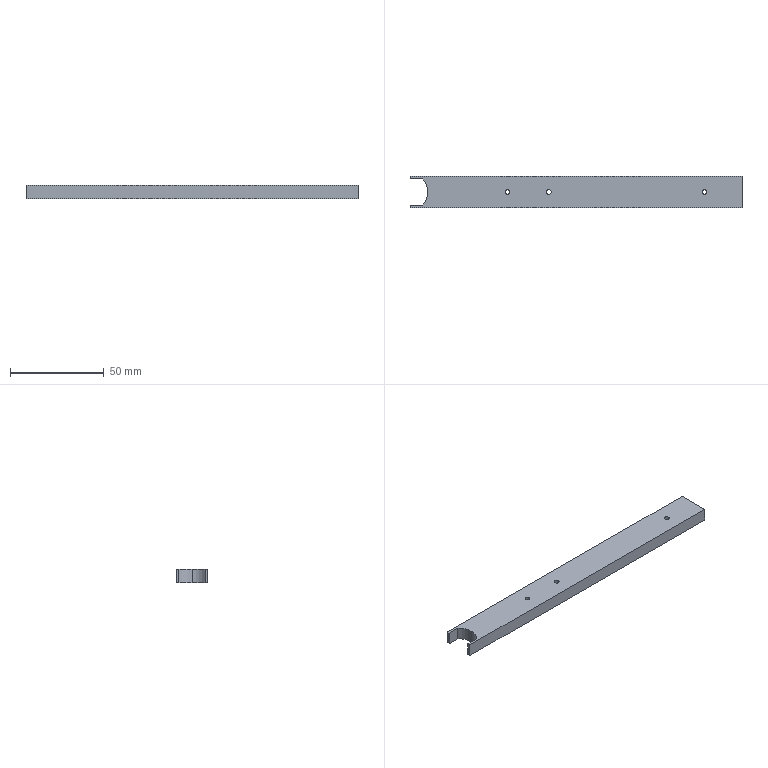Part | STEP file | BU-D02-2a#180 | 1 solid | 17 faces | box 177 x 17 x 7 mm | volume 20122 mm3 | plane 9 | cylinder 8 | commonest cylinder face diameters 2.5 x6 19 x2
STEP:
#1=CARTESIAN_POINT('',(0.,0.,0.));
#2=DIRECTION('',(0.,0.,1.));
#3=DIRECTION('',(1.,0.,0.));
#4=AXIS2_PLACEMENT_3D('',#1,#2,#3);
#5=CARTESIAN_POINT('',(53.25,0.,0.));
#6=VERTEX_POINT('',#5);
#7=CARTESIAN_POINT('',(53.25,0.,7.));
#8=VERTEX_POINT('',#7);
#9=CARTESIAN_POINT('',(53.25,0.,7.));
#10=DIRECTION('',(0.,0.,1.));
#11=VECTOR('',#10,1.);
#12=LINE('',#9,#11);
#13=CARTESIAN_POINT('',(52.,0.,7.));
#14=DIRECTION('',(0.,0.,1.));
#15=DIRECTION('',(1.,0.,0.));
#16=AXIS2_PLACEMENT_3D('',#13,#14,#15);
#17=CYLINDRICAL_SURFACE('',#16,1.25);
#18=CARTESIAN_POINT('',(6.283,0.));
#19=DIRECTION('',(0.,1.));
#20=VECTOR('',#19,1.);
#21=LINE('',#18,#20);
#22=(GEOMETRIC_REPRESENTATION_CONTEXT(2)PARAMETRIC_REPRESENTATION_CONTEXT()REPRESENTATION_CONTEXT('',''));
#23=DEFINITIONAL_REPRESENTATION('',(#21),#22);
#24=PCURVE('',#17,#23);
#25=CARTESIAN_POINT('',(52.,0.,7.));
#26=DIRECTION('',(0.,0.,1.));
#27=DIRECTION('',(1.,0.,0.));
#28=AXIS2_PLACEMENT_3D('',#25,#26,#27);
#29=CYLINDRICAL_SURFACE('',#28,1.25);
#30=CARTESIAN_POINT('',(0.,0.));
#31=DIRECTION('',(0.,1.));
#32=VECTOR('',#31,1.);
#33=LINE('',#30,#32);
#34=(GEOMETRIC_REPRESENTATION_CONTEXT(2)PARAMETRIC_REPRESENTATION_CONTEXT()REPRESENTATION_CONTEXT('',''));
#35=DEFINITIONAL_REPRESENTATION('',(#33),#34);
#36=PCURVE('',#29,#35);
#37=SURFACE_CURVE('',#12,(#24,#36),.PCURVE_S1.);
#38=EDGE_CURVE('',#6,#8,#37,.T.);
#39=ORIENTED_EDGE('',*,*,#38,.T.);
#40=CARTESIAN_POINT('',(50.75,0.,7.));
#41=VERTEX_POINT('',#40);
#42=CARTESIAN_POINT('',(52.,0.,7.));
#43=DIRECTION('',(0.,0.,1.));
#44=DIRECTION('',(1.,0.,0.));
#45=AXIS2_PLACEMENT_3D('',#42,#43,#44);
#46=CIRCLE('',#45,1.25);
#47=CARTESIAN_POINT('',(0.,0.));
#48=DIRECTION('',(1.,0.));
#49=VECTOR('',#48,1.);
#50=LINE('',#47,#49);
#51=(GEOMETRIC_REPRESENTATION_CONTEXT(2)PARAMETRIC_REPRESENTATION_CONTEXT()REPRESENTATION_CONTEXT('',''));
#52=DEFINITIONAL_REPRESENTATION('',(#50),#51);
#53=PCURVE('',#17,#52);
#54=CARTESIAN_POINT('',(0.,0.,7.));
#55=DIRECTION('',(0.,0.,1.));
#56=DIRECTION('',(1.,0.,0.));
#57=AXIS2_PLACEMENT_3D('',#54,#55,#56);
#58=PLANE('',#57);
#59=CARTESIAN_POINT('',(52.,0.));
#60=DIRECTION('',(1.,0.));
#61=AXIS2_PLACEMENT_2D('',#59,#60);
#62=CIRCLE('',#61,1.25);
#63=(GEOMETRIC_REPRESENTATION_CONTEXT(2)PARAMETRIC_REPRESENTATION_CONTEXT()REPRESENTATION_CONTEXT('',''));
#64=DEFINITIONAL_REPRESENTATION('',(#62),#63);
#65=PCURVE('',#58,#64);
#66=SURFACE_CURVE('',#46,(#53,#65),.PCURVE_S1.);
#67=EDGE_CURVE('',#41,#8,#66,.T.);
#68=ORIENTED_EDGE('',*,*,#67,.F.);
#69=CARTESIAN_POINT('',(50.75,0.,0.));
#70=VERTEX_POINT('',#69);
#71=CARTESIAN_POINT('',(50.75,0.,7.));
#72=DIRECTION('',(0.,0.,1.));
#73=VECTOR('',#72,1.);
#74=LINE('',#71,#73);
#75=CARTESIAN_POINT('',(3.142,0.));
#76=DIRECTION('',(0.,1.));
#77=VECTOR('',#76,1.);
#78=LINE('',#75,#77);
#79=(GEOMETRIC_REPRESENTATION_CONTEXT(2)PARAMETRIC_REPRESENTATION_CONTEXT()REPRESENTATION_CONTEXT('',''));
#80=DEFINITIONAL_REPRESENTATION('',(#78),#79);
#81=PCURVE('',#17,#80);
#82=CARTESIAN_POINT('',(3.142,0.));
#83=DIRECTION('',(0.,1.));
#84=VECTOR('',#83,1.);
#85=LINE('',#82,#84);
#86=(GEOMETRIC_REPRESENTATION_CONTEXT(2)PARAMETRIC_REPRESENTATION_CONTEXT()REPRESENTATION_CONTEXT('',''));
#87=DEFINITIONAL_REPRESENTATION('',(#85),#86);
#88=PCURVE('',#29,#87);
#89=SURFACE_CURVE('',#74,(#81,#88),.PCURVE_S1.);
#90=EDGE_CURVE('',#70,#41,#89,.T.);
#91=ORIENTED_EDGE('',*,*,#90,.F.);
#92=CARTESIAN_POINT('',(52.,0.,0.));
#93=DIRECTION('',(0.,0.,1.));
#94=DIRECTION('',(1.,0.,0.));
#95=AXIS2_PLACEMENT_3D('',#92,#93,#94);
#96=CIRCLE('',#95,1.25);
#97=CARTESIAN_POINT('',(0.,-7.));
#98=DIRECTION('',(1.,0.));
#99=VECTOR('',#98,1.);
#100=LINE('',#97,#99);
#101=(GEOMETRIC_REPRESENTATION_CONTEXT(2)PARAMETRIC_REPRESENTATION_CONTEXT()REPRESENTATION_CONTEXT('',''));
#102=DEFINITIONAL_REPRESENTATION('',(#100),#101);
#103=PCURVE('',#17,#102);
#104=CARTESIAN_POINT('',(0.,0.,0.));
#105=DIRECTION('',(0.,0.,1.));
#106=DIRECTION('',(1.,0.,0.));
#107=AXIS2_PLACEMENT_3D('',#104,#105,#106);
#108=PLANE('',#107);
#109=CARTESIAN_POINT('',(52.,0.));
#110=DIRECTION('',(1.,0.));
#111=AXIS2_PLACEMENT_2D('',#109,#110);
#112=CIRCLE('',#111,1.25);
#113=(GEOMETRIC_REPRESENTATION_CONTEXT(2)PARAMETRIC_REPRESENTATION_CONTEXT()REPRESENTATION_CONTEXT('',''));
#114=DEFINITIONAL_REPRESENTATION('',(#112),#113);
#115=PCURVE('',#108,#114);
#116=SURFACE_CURVE('',#96,(#103,#115),.PCURVE_S1.);
#117=EDGE_CURVE('',#70,#6,#116,.T.);
#118=ORIENTED_EDGE('',*,*,#117,.T.);
#119=EDGE_LOOP('',(#39,#68,#91,#118));
#120=FACE_BOUND('',#119,.F.);
#121=ADVANCED_FACE('',(#120),#17,.F.);
#122=CARTESIAN_POINT('',(75.25,0.,0.));
#123=VERTEX_POINT('',#122);
#124=CARTESIAN_POINT('',(75.25,0.,7.));
#125=VERTEX_POINT('',#124);
#126=CARTESIAN_POINT('',(75.25,0.,7.));
#127=DIRECTION('',(0.,0.,1.));
#128=VECTOR('',#127,1.);
#129=LINE('',#126,#128);
#130=CARTESIAN_POINT('',(74.,0.,7.));
#131=DIRECTION('',(0.,0.,1.));
#132=DIRECTION('',(1.,0.,0.));
#133=AXIS2_PLACEMENT_3D('',#130,#131,#132);
#134=CYLINDRICAL_SURFACE('',#133,1.25);
#135=CARTESIAN_POINT('',(6.283,0.));
#136=DIRECTION('',(0.,1.));
#137=VECTOR('',#136,1.);
#138=LINE('',#135,#137);
#139=(GEOMETRIC_REPRESENTATION_CONTEXT(2)PARAMETRIC_REPRESENTATION_CONTEXT()REPRESENTATION_CONTEXT('',''));
#140=DEFINITIONAL_REPRESENTATION('',(#138),#139);
#141=PCURVE('',#134,#140);
#142=CARTESIAN_POINT('',(74.,0.,7.));
#143=DIRECTION('',(0.,0.,1.));
#144=DIRECTION('',(1.,0.,0.));
#145=AXIS2_PLACEMENT_3D('',#142,#143,#144);
#146=CYLINDRICAL_SURFACE('',#145,1.25);
#147=CARTESIAN_POINT('',(0.,0.));
#148=DIRECTION('',(0.,1.));
#149=VECTOR('',#148,1.);
#150=LINE('',#147,#149);
#151=(GEOMETRIC_REPRESENTATION_CONTEXT(2)PARAMETRIC_REPRESENTATION_CONTEXT()REPRESENTATION_CONTEXT('',''));
#152=DEFINITIONAL_REPRESENTATION('',(#150),#151);
#153=PCURVE('',#146,#152);
#154=SURFACE_CURVE('',#129,(#141,#153),.PCURVE_S1.);
#155=EDGE_CURVE('',#123,#125,#154,.T.);
#156=ORIENTED_EDGE('',*,*,#155,.T.);
#157=CARTESIAN_POINT('',(72.75,0.,7.));
#158=VERTEX_POINT('',#157);
#159=CARTESIAN_POINT('',(74.,0.,7.));
#160=DIRECTION('',(0.,0.,1.));
#161=DIRECTION('',(1.,0.,0.));
#162=AXIS2_PLACEMENT_3D('',#159,#160,#161);
#163=CIRCLE('',#162,1.25);
#164=CARTESIAN_POINT('',(0.,0.));
#165=DIRECTION('',(1.,0.));
#166=VECTOR('',#165,1.);
#167=LINE('',#164,#166);
#168=(GEOMETRIC_REPRESENTATION_CONTEXT(2)PARAMETRIC_REPRESENTATION_CONTEXT()REPRESENTATION_CONTEXT('',''));
#169=DEFINITIONAL_REPRESENTATION('',(#167),#168);
#170=PCURVE('',#134,#169);
#171=CARTESIAN_POINT('',(74.,0.));
#172=DIRECTION('',(1.,0.));
#173=AXIS2_PLACEMENT_2D('',#171,#172);
#174=CIRCLE('',#173,1.25);
#175=(GEOMETRIC_REPRESENTATION_CONTEXT(2)PARAMETRIC_REPRESENTATION_CONTEXT()REPRESENTATION_CONTEXT('',''));
#176=DEFINITIONAL_REPRESENTATION('',(#174),#175);
#177=PCURVE('',#58,#176);
#178=SURFACE_CURVE('',#163,(#170,#177),.PCURVE_S1.);
#179=EDGE_CURVE('',#158,#125,#178,.T.);
#180=ORIENTED_EDGE('',*,*,#179,.F.);
#181=CARTESIAN_POINT('',(72.75,0.,0.));
#182=VERTEX_POINT('',#181);
#183=CARTESIAN_POINT('',(72.75,0.,7.));
#184=DIRECTION('',(0.,0.,1.));
#185=VECTOR('',#184,1.);
#186=LINE('',#183,#185);
#187=CARTESIAN_POINT('',(3.142,0.));
#188=DIRECTION('',(0.,1.));
#189=VECTOR('',#188,1.);
#190=LINE('',#187,#189);
#191=(GEOMETRIC_REPRESENTATION_CONTEXT(2)PARAMETRIC_REPRESENTATION_CONTEXT()REPRESENTATION_CONTEXT('',''));
#192=DEFINITIONAL_REPRESENTATION('',(#190),#191);
#193=PCURVE('',#134,#192);
#194=CARTESIAN_POINT('',(3.142,0.));
#195=DIRECTION('',(0.,1.));
#196=VECTOR('',#195,1.);
#197=LINE('',#194,#196);
#198=(GEOMETRIC_REPRESENTATION_CONTEXT(2)PARAMETRIC_REPRESENTATION_CONTEXT()REPRESENTATION_CONTEXT('',''));
#199=DEFINITIONAL_REPRESENTATION('',(#197),#198);
#200=PCURVE('',#146,#199);
#201=SURFACE_CURVE('',#186,(#193,#200),.PCURVE_S1.);
#202=EDGE_CURVE('',#182,#158,#201,.T.);
#203=ORIENTED_EDGE('',*,*,#202,.F.);
#204=CARTESIAN_POINT('',(74.,0.,0.));
#205=DIRECTION('',(0.,0.,1.));
#206=DIRECTION('',(1.,0.,0.));
#207=AXIS2_PLACEMENT_3D('',#204,#205,#206);
#208=CIRCLE('',#207,1.25);
#209=CARTESIAN_POINT('',(0.,-7.));
#210=DIRECTION('',(1.,0.));
#211=VECTOR('',#210,1.);
#212=LINE('',#209,#211);
#213=(GEOMETRIC_REPRESENTATION_CONTEXT(2)PARAMETRIC_REPRESENTATION_CONTEXT()REPRESENTATION_CONTEXT('',''));
#214=DEFINITIONAL_REPRESENTATION('',(#212),#213);
#215=PCURVE('',#134,#214);
#216=CARTESIAN_POINT('',(74.,0.));
#217=DIRECTION('',(1.,0.));
#218=AXIS2_PLACEMENT_2D('',#216,#217);
#219=CIRCLE('',#218,1.25);
#220=(GEOMETRIC_REPRESENTATION_CONTEXT(2)PARAMETRIC_REPRESENTATION_CONTEXT()REPRESENTATION_CONTEXT('',''));
#221=DEFINITIONAL_REPRESENTATION('',(#219),#220);
#222=PCURVE('',#108,#221);
#223=SURFACE_CURVE('',#208,(#215,#222),.PCURVE_S1.);
#224=EDGE_CURVE('',#182,#123,#223,.T.);
#225=ORIENTED_EDGE('',*,*,#224,.T.);
#226=EDGE_LOOP('',(#156,#180,#203,#225));
#227=FACE_BOUND('',#226,.F.);
#228=ADVANCED_FACE('',(#227),#134,.F.);
#229=CARTESIAN_POINT('',(158.25,0.,0.));
#230=VERTEX_POINT('',#229);
#231=CARTESIAN_POINT('',(158.25,0.,7.));
#232=VERTEX_POINT('',#231);
#233=CARTESIAN_POINT('',(158.25,0.,7.));
#234=DIRECTION('',(0.,0.,1.));
#235=VECTOR('',#234,1.);
#236=LINE('',#233,#235);
#237=CARTESIAN_POINT('',(157.,0.,7.));
#238=DIRECTION('',(0.,0.,1.));
#239=DIRECTION('',(1.,0.,0.));
#240=AXIS2_PLACEMENT_3D('',#237,#238,#239);
#241=CYLINDRICAL_SURFACE('',#240,1.25);
#242=CARTESIAN_POINT('',(6.283,0.));
#243=DIRECTION('',(0.,1.));
#244=VECTOR('',#243,1.);
#245=LINE('',#242,#244);
#246=(GEOMETRIC_REPRESENTATION_CONTEXT(2)PARAMETRIC_REPRESENTATION_CONTEXT()REPRESENTATION_CONTEXT('',''));
#247=DEFINITIONAL_REPRESENTATION('',(#245),#246);
#248=PCURVE('',#241,#247);
#249=CARTESIAN_POINT('',(157.,0.,7.));
#250=DIRECTION('',(0.,0.,1.));
#251=DIRECTION('',(1.,0.,0.));
#252=AXIS2_PLACEMENT_3D('',#249,#250,#251);
#253=CYLINDRICAL_SURFACE('',#252,1.25);
#254=CARTESIAN_POINT('',(0.,0.));
#255=DIRECTION('',(0.,1.));
#256=VECTOR('',#255,1.);
#257=LINE('',#254,#256);
#258=(GEOMETRIC_REPRESENTATION_CONTEXT(2)PARAMETRIC_REPRESENTATION_CONTEXT()REPRESENTATION_CONTEXT('',''));
#259=DEFINITIONAL_REPRESENTATION('',(#257),#258);
#260=PCURVE('',#253,#259);
#261=SURFACE_CURVE('',#236,(#248,#260),.PCURVE_S1.);
#262=EDGE_CURVE('',#230,#232,#261,.T.);
#263=ORIENTED_EDGE('',*,*,#262,.T.);
#264=CARTESIAN_POINT('',(155.75,0.,7.));
#265=VERTEX_POINT('',#264);
#266=CARTESIAN_POINT('',(157.,0.,7.));
#267=DIRECTION('',(0.,0.,1.));
#268=DIRECTION('',(1.,0.,0.));
#269=AXIS2_PLACEMENT_3D('',#266,#267,#268);
#270=CIRCLE('',#269,1.25);
#271=CARTESIAN_POINT('',(0.,0.));
#272=DIRECTION('',(1.,0.));
#273=VECTOR('',#272,1.);
#274=LINE('',#271,#273);
#275=(GEOMETRIC_REPRESENTATION_CONTEXT(2)PARAMETRIC_REPRESENTATION_CONTEXT()REPRESENTATION_CONTEXT('',''));
#276=DEFINITIONAL_REPRESENTATION('',(#274),#275);
#277=PCURVE('',#241,#276);
#278=CARTESIAN_POINT('',(157.,0.));
#279=DIRECTION('',(1.,0.));
#280=AXIS2_PLACEMENT_2D('',#278,#279);
#281=CIRCLE('',#280,1.25);
#282=(GEOMETRIC_REPRESENTATION_CONTEXT(2)PARAMETRIC_REPRESENTATION_CONTEXT()REPRESENTATION_CONTEXT('',''));
#283=DEFINITIONAL_REPRESENTATION('',(#281),#282);
#284=PCURVE('',#58,#283);
#285=SURFACE_CURVE('',#270,(#277,#284),.PCURVE_S1.);
#286=EDGE_CURVE('',#265,#232,#285,.T.);
#287=ORIENTED_EDGE('',*,*,#286,.F.);
#288=CARTESIAN_POINT('',(155.75,0.,0.));
#289=VERTEX_POINT('',#288);
#290=CARTESIAN_POINT('',(155.75,0.,7.));
#291=DIRECTION('',(0.,0.,1.));
#292=VECTOR('',#291,1.);
#293=LINE('',#290,#292);
#294=CARTESIAN_POINT('',(3.142,0.));
#295=DIRECTION('',(0.,1.));
#296=VECTOR('',#295,1.);
#297=LINE('',#294,#296);
#298=(GEOMETRIC_REPRESENTATION_CONTEXT(2)PARAMETRIC_REPRESENTATION_CONTEXT()REPRESENTATION_CONTEXT('',''));
#299=DEFINITIONAL_REPRESENTATION('',(#297),#298);
#300=PCURVE('',#241,#299);
#301=CARTESIAN_POINT('',(3.142,0.));
#302=DIRECTION('',(0.,1.));
#303=VECTOR('',#302,1.);
#304=LINE('',#301,#303);
#305=(GEOMETRIC_REPRESENTATION_CONTEXT(2)PARAMETRIC_REPRESENTATION_CONTEXT()REPRESENTATION_CONTEXT('',''));
#306=DEFINITIONAL_REPRESENTATION('',(#304),#305);
#307=PCURVE('',#253,#306);
#308=SURFACE_CURVE('',#293,(#300,#307),.PCURVE_S1.);
#309=EDGE_CURVE('',#289,#265,#308,.T.);
#310=ORIENTED_EDGE('',*,*,#309,.F.);
#311=CARTESIAN_POINT('',(157.,0.,0.));
#312=DIRECTION('',(0.,0.,1.));
#313=DIRECTION('',(1.,0.,0.));
#314=AXIS2_PLACEMENT_3D('',#311,#312,#313);
#315=CIRCLE('',#314,1.25);
#316=CARTESIAN_POINT('',(0.,-7.));
#317=DIRECTION('',(1.,0.));
#318=VECTOR('',#317,1.);
#319=LINE('',#316,#318);
#320=(GEOMETRIC_REPRESENTATION_CONTEXT(2)PARAMETRIC_REPRESENTATION_CONTEXT()REPRESENTATION_CONTEXT('',''));
#321=DEFINITIONAL_REPRESENTATION('',(#319),#320);
#322=PCURVE('',#241,#321);
#323=CARTESIAN_POINT('',(157.,0.));
#324=DIRECTION('',(1.,0.));
#325=AXIS2_PLACEMENT_2D('',#323,#324);
#326=CIRCLE('',#325,1.25);
#327=(GEOMETRIC_REPRESENTATION_CONTEXT(2)PARAMETRIC_REPRESENTATION_CONTEXT()REPRESENTATION_CONTEXT('',''));
#328=DEFINITIONAL_REPRESENTATION('',(#326),#327);
#329=PCURVE('',#108,#328);
#330=SURFACE_CURVE('',#315,(#322,#329),.PCURVE_S1.);
#331=EDGE_CURVE('',#289,#230,#330,.T.);
#332=ORIENTED_EDGE('',*,*,#331,.T.);
#333=EDGE_LOOP('',(#263,#287,#310,#332));
#334=FACE_BOUND('',#333,.F.);
#335=ADVANCED_FACE('',(#334),#241,.F.);
#336=CARTESIAN_POINT('',(6.423,7.,0.));
#337=VERTEX_POINT('',#336);
#338=CARTESIAN_POINT('',(6.423,7.,7.));
#339=VERTEX_POINT('',#338);
#340=CARTESIAN_POINT('',(6.423,7.,0.));
#341=DIRECTION('',(0.,0.,1.));
#342=VECTOR('',#341,1.);
#343=LINE('',#340,#342);
#344=CARTESIAN_POINT('',(0.,0.,0.));
#345=DIRECTION('',(0.,0.,1.));
#346=DIRECTION('',(1.,0.,0.));
#347=AXIS2_PLACEMENT_3D('',#344,#345,#346);
#348=CYLINDRICAL_SURFACE('',#347,9.5);
#349=CARTESIAN_POINT('',(0.8284,0.));
#350=DIRECTION('',(0.,1.));
#351=VECTOR('',#350,1.);
#352=LINE('',#349,#351);
#353=(GEOMETRIC_REPRESENTATION_CONTEXT(2)PARAMETRIC_REPRESENTATION_CONTEXT()REPRESENTATION_CONTEXT('',''));
#354=DEFINITIONAL_REPRESENTATION('',(#352),#353);
#355=PCURVE('',#348,#354);
#356=CARTESIAN_POINT('',(0.,7.,0.));
#357=DIRECTION('',(0.,-1.,0.));
#358=DIRECTION('',(0.,0.,-1.));
#359=AXIS2_PLACEMENT_3D('',#356,#357,#358);
#360=PLANE('',#359);
#361=CARTESIAN_POINT('',(0.,6.423));
#362=DIRECTION('',(-1.,0.));
#363=VECTOR('',#362,1.);
#364=LINE('',#361,#363);
#365=(GEOMETRIC_REPRESENTATION_CONTEXT(2)PARAMETRIC_REPRESENTATION_CONTEXT()REPRESENTATION_CONTEXT('',''));
#366=DEFINITIONAL_REPRESENTATION('',(#364),#365);
#367=PCURVE('',#360,#366);
#368=SURFACE_CURVE('',#343,(#355,#367),.PCURVE_S1.);
#369=EDGE_CURVE('',#337,#339,#368,.T.);
#370=ORIENTED_EDGE('',*,*,#369,.T.);
#371=CARTESIAN_POINT('',(9.5,0.,7.));
#372=VERTEX_POINT('',#371);
#373=CARTESIAN_POINT('',(0.,0.,7.));
#374=DIRECTION('',(0.,0.,-1.));
#375=DIRECTION('',(1.,0.,0.));
#376=AXIS2_PLACEMENT_3D('',#373,#374,#375);
#377=CIRCLE('',#376,9.5);
#378=CARTESIAN_POINT('',(6.283,7.));
#379=DIRECTION('',(-1.,0.));
#380=VECTOR('',#379,1.);
#381=LINE('',#378,#380);
#382=(GEOMETRIC_REPRESENTATION_CONTEXT(2)PARAMETRIC_REPRESENTATION_CONTEXT()REPRESENTATION_CONTEXT('',''));
#383=DEFINITIONAL_REPRESENTATION('',(#381),#382);
#384=PCURVE('',#348,#383);
#385=CARTESIAN_POINT('',(9.5,0.));
#386=CARTESIAN_POINT('',(9.5,-16.454));
#387=CARTESIAN_POINT('',(-4.75,-8.227));
#388=CARTESIAN_POINT('',(-19.,0.));
#389=CARTESIAN_POINT('',(-4.75,8.227));
#390=CARTESIAN_POINT('',(9.5,16.454));
#391=CARTESIAN_POINT('',(9.5,0.));
#392=(BOUNDED_CURVE()B_SPLINE_CURVE(2,(#385,#386,#387,#388,#389,#390,#391),.UNSPECIFIED.,.T.,.F.)B_SPLINE_CURVE_WITH_KNOTS((1,2,2,2,2,1),(-2.094,0.,2.094,4.189,6.283,8.378),.UNSPECIFIED.)CURVE()GEOMETRIC_REPRESENTATION_ITEM()RATIONAL_B_SPLINE_CURVE((1.,0.5,1.,0.5,1.,0.5,1.))REPRESENTATION_ITEM(''));
#393=(GEOMETRIC_REPRESENTATION_CONTEXT(2)PARAMETRIC_REPRESENTATION_CONTEXT()REPRESENTATION_CONTEXT('',''));
#394=DEFINITIONAL_REPRESENTATION('',(#392),#393);
#395=PCURVE('',#58,#394);
#396=SURFACE_CURVE('',#377,(#384,#395),.PCURVE_S1.);
#397=EDGE_CURVE('',#339,#372,#396,.T.);
#398=ORIENTED_EDGE('',*,*,#397,.T.);
#399=CARTESIAN_POINT('',(9.5,0.,0.));
#400=VERTEX_POINT('',#399);
#401=CARTESIAN_POINT('',(9.5,0.,0.));
#402=DIRECTION('',(0.,0.,1.));
#403=VECTOR('',#402,1.);
#404=LINE('',#401,#403);
#405=CARTESIAN_POINT('',(0.,0.));
#406=DIRECTION('',(0.,1.));
#407=VECTOR('',#406,1.);
#408=LINE('',#405,#407);
#409=(GEOMETRIC_REPRESENTATION_CONTEXT(2)PARAMETRIC_REPRESENTATION_CONTEXT()REPRESENTATION_CONTEXT('',''));
#410=DEFINITIONAL_REPRESENTATION('',(#408),#409);
#411=PCURVE('',#348,#410);
#412=CARTESIAN_POINT('',(0.,0.,0.));
#413=DIRECTION('',(0.,0.,1.));
#414=DIRECTION('',(1.,0.,0.));
#415=AXIS2_PLACEMENT_3D('',#412,#413,#414);
#416=CYLINDRICAL_SURFACE('',#415,9.5);
#417=CARTESIAN_POINT('',(6.283,0.));
#418=DIRECTION('',(0.,1.));
#419=VECTOR('',#418,1.);
#420=LINE('',#417,#419);
#421=(GEOMETRIC_REPRESENTATION_CONTEXT(2)PARAMETRIC_REPRESENTATION_CONTEXT()REPRESENTATION_CONTEXT('',''));
#422=DEFINITIONAL_REPRESENTATION('',(#420),#421);
#423=PCURVE('',#416,#422);
#424=SURFACE_CURVE('',#404,(#411,#423),.PCURVE_S1.);
#425=EDGE_CURVE('',#400,#372,#424,.T.);
#426=ORIENTED_EDGE('',*,*,#425,.F.);
#427=CARTESIAN_POINT('',(0.,0.,0.));
#428=DIRECTION('',(0.,0.,-1.));
#429=DIRECTION('',(1.,0.,0.));
#430=AXIS2_PLACEMENT_3D('',#427,#428,#429);
#431=CIRCLE('',#430,9.5);
#432=CARTESIAN_POINT('',(6.283,0.));
#433=DIRECTION('',(-1.,0.));
#434=VECTOR('',#433,1.);
#435=LINE('',#432,#434);
#436=(GEOMETRIC_REPRESENTATION_CONTEXT(2)PARAMETRIC_REPRESENTATION_CONTEXT()REPRESENTATION_CONTEXT('',''));
#437=DEFINITIONAL_REPRESENTATION('',(#435),#436);
#438=PCURVE('',#348,#437);
#439=CARTESIAN_POINT('',(9.5,0.));
#440=CARTESIAN_POINT('',(9.5,-16.454));
#441=CARTESIAN_POINT('',(-4.75,-8.227));
#442=CARTESIAN_POINT('',(-19.,0.));
#443=CARTESIAN_POINT('',(-4.75,8.227));
#444=CARTESIAN_POINT('',(9.5,16.454));
#445=CARTESIAN_POINT('',(9.5,0.));
#446=(BOUNDED_CURVE()B_SPLINE_CURVE(2,(#439,#440,#441,#442,#443,#444,#445),.UNSPECIFIED.,.T.,.F.)B_SPLINE_CURVE_WITH_KNOTS((1,2,2,2,2,1),(-2.094,0.,2.094,4.189,6.283,8.378),.UNSPECIFIED.)CURVE()GEOMETRIC_REPRESENTATION_ITEM()RATIONAL_B_SPLINE_CURVE((1.,0.5,1.,0.5,1.,0.5,1.))REPRESENTATION_ITEM(''));
#447=(GEOMETRIC_REPRESENTATION_CONTEXT(2)PARAMETRIC_REPRESENTATION_CONTEXT()REPRESENTATION_CONTEXT('',''));
#448=DEFINITIONAL_REPRESENTATION('',(#446),#447);
#449=PCURVE('',#108,#448);
#450=SURFACE_CURVE('',#431,(#438,#449),.PCURVE_S1.);
#451=EDGE_CURVE('',#337,#400,#450,.T.);
#452=ORIENTED_EDGE('',*,*,#451,.F.);
#453=EDGE_LOOP('',(#370,#398,#426,#452));
#454=FACE_BOUND('',#453,.F.);
#455=ADVANCED_FACE('',(#454),#348,.F.);
#456=CARTESIAN_POINT('',(177.,-8.5,0.));
#457=VERTEX_POINT('',#456);
#458=CARTESIAN_POINT('',(177.,8.5,0.));
#459=VERTEX_POINT('',#458);
#460=CARTESIAN_POINT('',(177.,7.5,0.));
#461=DIRECTION('',(0.,1.,0.));
#462=VECTOR('',#461,1.);
#463=LINE('',#460,#462);
#464=CARTESIAN_POINT('',(177.,7.5,7.));
#465=DIRECTION('',(-1.,0.,0.));
#466=DIRECTION('',(0.,0.,1.));
#467=AXIS2_PLACEMENT_3D('',#464,#465,#466);
#468=PLANE('',#467);
#469=CARTESIAN_POINT('',(-7.,0.));
#470=DIRECTION('',(0.,1.));
#471=VECTOR('',#470,1.);
#472=LINE('',#469,#471);
#473=(GEOMETRIC_REPRESENTATION_CONTEXT(2)PARAMETRIC_REPRESENTATION_CONTEXT()REPRESENTATION_CONTEXT('',''));
#474=DEFINITIONAL_REPRESENTATION('',(#472),#473);
#475=PCURVE('',#468,#474);
#476=CARTESIAN_POINT('',(177.,7.5));
#477=DIRECTION('',(0.,1.));
#478=VECTOR('',#477,1.);
#479=LINE('',#476,#478);
#480=(GEOMETRIC_REPRESENTATION_CONTEXT(2)PARAMETRIC_REPRESENTATION_CONTEXT()REPRESENTATION_CONTEXT('',''));
#481=DEFINITIONAL_REPRESENTATION('',(#479),#480);
#482=PCURVE('',#108,#481);
#483=SURFACE_CURVE('',#463,(#475,#482),.PCURVE_S1.);
#484=EDGE_CURVE('',#457,#459,#483,.T.);
#485=ORIENTED_EDGE('',*,*,#484,.T.);
#486=CARTESIAN_POINT('',(177.,8.5,7.));
#487=VERTEX_POINT('',#486);
#488=CARTESIAN_POINT('',(177.,8.5,0.));
#489=DIRECTION('',(0.,0.,-1.));
#490=VECTOR('',#489,1.);
#491=LINE('',#488,#490);
#492=CARTESIAN_POINT('',(-7.,1.));
#493=DIRECTION('',(-1.,0.));
#494=VECTOR('',#493,1.);
#495=LINE('',#492,#494);
#496=(GEOMETRIC_REPRESENTATION_CONTEXT(2)PARAMETRIC_REPRESENTATION_CONTEXT()REPRESENTATION_CONTEXT('',''));
#497=DEFINITIONAL_REPRESENTATION('',(#495),#496);
#498=PCURVE('',#468,#497);
#499=CARTESIAN_POINT('',(0.,8.5,7.));
#500=DIRECTION('',(0.,1.,0.));
#501=DIRECTION('',(0.,0.,1.));
#502=AXIS2_PLACEMENT_3D('',#499,#500,#501);
#503=PLANE('',#502);
#504=CARTESIAN_POINT('',(-7.,177.));
#505=DIRECTION('',(-1.,0.));
#506=VECTOR('',#505,1.);
#507=LINE('',#504,#506);
#508=(GEOMETRIC_REPRESENTATION_CONTEXT(2)PARAMETRIC_REPRESENTATION_CONTEXT()REPRESENTATION_CONTEXT('',''));
#509=DEFINITIONAL_REPRESENTATION('',(#507),#508);
#510=PCURVE('',#503,#509);
#511=SURFACE_CURVE('',#491,(#498,#510),.PCURVE_S1.);
#512=EDGE_CURVE('',#487,#459,#511,.T.);
#513=ORIENTED_EDGE('',*,*,#512,.F.);
#514=CARTESIAN_POINT('',(177.,-8.5,7.));
#515=VERTEX_POINT('',#514);
#516=CARTESIAN_POINT('',(177.,7.5,7.));
#517=DIRECTION('',(0.,1.,0.));
#518=VECTOR('',#517,1.);
#519=LINE('',#516,#518);
#520=CARTESIAN_POINT('',(0.,0.));
#521=DIRECTION('',(0.,1.));
#522=VECTOR('',#521,1.);
#523=LINE('',#520,#522);
#524=(GEOMETRIC_REPRESENTATION_CONTEXT(2)PARAMETRIC_REPRESENTATION_CONTEXT()REPRESENTATION_CONTEXT('',''));
#525=DEFINITIONAL_REPRESENTATION('',(#523),#524);
#526=PCURVE('',#468,#525);
#527=CARTESIAN_POINT('',(177.,7.5));
#528=DIRECTION('',(0.,1.));
#529=VECTOR('',#528,1.);
#530=LINE('',#527,#529);
#531=(GEOMETRIC_REPRESENTATION_CONTEXT(2)PARAMETRIC_REPRESENTATION_CONTEXT()REPRESENTATION_CONTEXT('',''));
#532=DEFINITIONAL_REPRESENTATION('',(#530),#531);
#533=PCURVE('',#58,#532);
#534=SURFACE_CURVE('',#519,(#526,#533),.PCURVE_S1.);
#535=EDGE_CURVE('',#515,#487,#534,.T.);
#536=ORIENTED_EDGE('',*,*,#535,.F.);
#537=CARTESIAN_POINT('',(177.,-8.5,0.));
#538=DIRECTION('',(0.,0.,1.));
#539=VECTOR('',#538,1.);
#540=LINE('',#537,#539);
#541=CARTESIAN_POINT('',(-7.,-16.));
#542=DIRECTION('',(1.,0.));
#543=VECTOR('',#542,1.);
#544=LINE('',#541,#543);
#545=(GEOMETRIC_REPRESENTATION_CONTEXT(2)PARAMETRIC_REPRESENTATION_CONTEXT()REPRESENTATION_CONTEXT('',''));
#546=DEFINITIONAL_REPRESENTATION('',(#544),#545);
#547=PCURVE('',#468,#546);
#548=CARTESIAN_POINT('',(0.,-8.5,7.));
#549=DIRECTION('',(0.,1.,0.));
#550=DIRECTION('',(0.,0.,1.));
#551=AXIS2_PLACEMENT_3D('',#548,#549,#550);
#552=PLANE('',#551);
#553=CARTESIAN_POINT('',(-7.,177.));
#554=DIRECTION('',(1.,0.));
#555=VECTOR('',#554,1.);
#556=LINE('',#553,#555);
#557=(GEOMETRIC_REPRESENTATION_CONTEXT(2)PARAMETRIC_REPRESENTATION_CONTEXT()REPRESENTATION_CONTEXT('',''));
#558=DEFINITIONAL_REPRESENTATION('',(#556),#557);
#559=PCURVE('',#552,#558);
#560=SURFACE_CURVE('',#540,(#547,#559),.PCURVE_S1.);
#561=EDGE_CURVE('',#457,#515,#560,.T.);
#562=ORIENTED_EDGE('',*,*,#561,.F.);
#563=EDGE_LOOP('',(#485,#513,#536,#562));
#564=FACE_BOUND('',#563,.T.);
#565=ADVANCED_FACE('',(#564),#468,.F.);
#566=CARTESIAN_POINT('',(52.,0.,7.));
#567=DIRECTION('',(0.,0.,1.));
#568=DIRECTION('',(1.,0.,0.));
#569=AXIS2_PLACEMENT_3D('',#566,#567,#568);
#570=CIRCLE('',#569,1.25);
#571=CARTESIAN_POINT('',(52.,0.));
#572=DIRECTION('',(1.,0.));
#573=AXIS2_PLACEMENT_2D('',#571,#572);
#574=CIRCLE('',#573,1.25);
#575=(GEOMETRIC_REPRESENTATION_CONTEXT(2)PARAMETRIC_REPRESENTATION_CONTEXT()REPRESENTATION_CONTEXT('',''));
#576=DEFINITIONAL_REPRESENTATION('',(#574),#575);
#577=PCURVE('',#58,#576);
#578=CARTESIAN_POINT('',(0.,0.));
#579=DIRECTION('',(1.,0.));
#580=VECTOR('',#579,1.);
#581=LINE('',#578,#580);
#582=(GEOMETRIC_REPRESENTATION_CONTEXT(2)PARAMETRIC_REPRESENTATION_CONTEXT()REPRESENTATION_CONTEXT('',''));
#583=DEFINITIONAL_REPRESENTATION('',(#581),#582);
#584=PCURVE('',#29,#583);
#585=SURFACE_CURVE('',#570,(#577,#584),.PCURVE_S1.);
#586=EDGE_CURVE('',#8,#41,#585,.T.);
#587=ORIENTED_EDGE('',*,*,#586,.F.);
#588=ORIENTED_EDGE('',*,*,#67,.F.);
#589=EDGE_LOOP('',(#587,#588));
#590=FACE_BOUND('',#589,.T.);
#591=CARTESIAN_POINT('',(74.,0.,7.));
#592=DIRECTION('',(0.,0.,1.));
#593=DIRECTION('',(1.,0.,0.));
#594=AXIS2_PLACEMENT_3D('',#591,#592,#593);
#595=CIRCLE('',#594,1.25);
#596=CARTESIAN_POINT('',(74.,0.));
#597=DIRECTION('',(1.,0.));
#598=AXIS2_PLACEMENT_2D('',#596,#597);
#599=CIRCLE('',#598,1.25);
#600=(GEOMETRIC_REPRESENTATION_CONTEXT(2)PARAMETRIC_REPRESENTATION_CONTEXT()REPRESENTATION_CONTEXT('',''));
#601=DEFINITIONAL_REPRESENTATION('',(#599),#600);
#602=PCURVE('',#58,#601);
#603=CARTESIAN_POINT('',(0.,0.));
#604=DIRECTION('',(1.,0.));
#605=VECTOR('',#604,1.);
#606=LINE('',#603,#605);
#607=(GEOMETRIC_REPRESENTATION_CONTEXT(2)PARAMETRIC_REPRESENTATION_CONTEXT()REPRESENTATION_CONTEXT('',''));
#608=DEFINITIONAL_REPRESENTATION('',(#606),#607);
#609=PCURVE('',#146,#608);
#610=SURFACE_CURVE('',#595,(#602,#609),.PCURVE_S1.);
#611=EDGE_CURVE('',#125,#158,#610,.T.);
#612=ORIENTED_EDGE('',*,*,#611,.F.);
#613=ORIENTED_EDGE('',*,*,#179,.F.);
#614=EDGE_LOOP('',(#612,#613));
#615=FACE_BOUND('',#614,.T.);
#616=CARTESIAN_POINT('',(157.,0.,7.));
#617=DIRECTION('',(0.,0.,1.));
#618=DIRECTION('',(1.,0.,0.));
#619=AXIS2_PLACEMENT_3D('',#616,#617,#618);
#620=CIRCLE('',#619,1.25);
#621=CARTESIAN_POINT('',(157.,0.));
#622=DIRECTION('',(1.,0.));
#623=AXIS2_PLACEMENT_2D('',#621,#622);
#624=CIRCLE('',#623,1.25);
#625=(GEOMETRIC_REPRESENTATION_CONTEXT(2)PARAMETRIC_REPRESENTATION_CONTEXT()REPRESENTATION_CONTEXT('',''));
#626=DEFINITIONAL_REPRESENTATION('',(#624),#625);
#627=PCURVE('',#58,#626);
#628=CARTESIAN_POINT('',(0.,0.));
#629=DIRECTION('',(1.,0.));
#630=VECTOR('',#629,1.);
#631=LINE('',#628,#630);
#632=(GEOMETRIC_REPRESENTATION_CONTEXT(2)PARAMETRIC_REPRESENTATION_CONTEXT()REPRESENTATION_CONTEXT('',''));
#633=DEFINITIONAL_REPRESENTATION('',(#631),#632);
#634=PCURVE('',#253,#633);
#635=SURFACE_CURVE('',#620,(#627,#634),.PCURVE_S1.);
#636=EDGE_CURVE('',#232,#265,#635,.T.);
#637=ORIENTED_EDGE('',*,*,#636,.F.);
#638=ORIENTED_EDGE('',*,*,#286,.F.);
#639=EDGE_LOOP('',(#637,#638));
#640=FACE_BOUND('',#639,.T.);
#641=ORIENTED_EDGE('',*,*,#535,.T.);
#642=CARTESIAN_POINT('',(0.,8.5,7.));
#643=VERTEX_POINT('',#642);
#644=CARTESIAN_POINT('',(0.,8.5,7.));
#645=DIRECTION('',(1.,0.,0.));
#646=VECTOR('',#645,1.);
#647=LINE('',#644,#646);
#648=CARTESIAN_POINT('',(0.,8.5));
#649=DIRECTION('',(1.,0.));
#650=VECTOR('',#649,1.);
#651=LINE('',#648,#650);
#652=(GEOMETRIC_REPRESENTATION_CONTEXT(2)PARAMETRIC_REPRESENTATION_CONTEXT()REPRESENTATION_CONTEXT('',''));
#653=DEFINITIONAL_REPRESENTATION('',(#651),#652);
#654=PCURVE('',#58,#653);
#655=CARTESIAN_POINT('',(0.,0.));
#656=DIRECTION('',(0.,1.));
#657=VECTOR('',#656,1.);
#658=LINE('',#655,#657);
#659=(GEOMETRIC_REPRESENTATION_CONTEXT(2)PARAMETRIC_REPRESENTATION_CONTEXT()REPRESENTATION_CONTEXT('',''));
#660=DEFINITIONAL_REPRESENTATION('',(#658),#659);
#661=PCURVE('',#503,#660);
#662=SURFACE_CURVE('',#647,(#654,#661),.PCURVE_S1.);
#663=EDGE_CURVE('',#643,#487,#662,.T.);
#664=ORIENTED_EDGE('',*,*,#663,.F.);
#665=CARTESIAN_POINT('',(0.,7.,7.));
#666=VERTEX_POINT('',#665);
#667=CARTESIAN_POINT('',(0.,7.5,7.));
#668=DIRECTION('',(0.,-1.,0.));
#669=VECTOR('',#668,1.);
#670=LINE('',#667,#669);
#671=CARTESIAN_POINT('',(0.,7.5));
#672=DIRECTION('',(0.,-1.));
#673=VECTOR('',#672,1.);
#674=LINE('',#671,#673);
#675=(GEOMETRIC_REPRESENTATION_CONTEXT(2)PARAMETRIC_REPRESENTATION_CONTEXT()REPRESENTATION_CONTEXT('',''));
#676=DEFINITIONAL_REPRESENTATION('',(#674),#675);
#677=PCURVE('',#58,#676);
#678=CARTESIAN_POINT('',(0.,7.5,0.));
#679=DIRECTION('',(-1.,0.,0.));
#680=DIRECTION('',(0.,0.,1.));
#681=AXIS2_PLACEMENT_3D('',#678,#679,#680);
#682=PLANE('',#681);
#683=CARTESIAN_POINT('',(7.,0.));
#684=DIRECTION('',(0.,-1.));
#685=VECTOR('',#684,1.);
#686=LINE('',#683,#685);
#687=(GEOMETRIC_REPRESENTATION_CONTEXT(2)PARAMETRIC_REPRESENTATION_CONTEXT()REPRESENTATION_CONTEXT('',''));
#688=DEFINITIONAL_REPRESENTATION('',(#686),#687);
#689=PCURVE('',#682,#688);
#690=SURFACE_CURVE('',#670,(#677,#689),.PCURVE_S1.);
#691=EDGE_CURVE('',#643,#666,#690,.T.);
#692=ORIENTED_EDGE('',*,*,#691,.T.);
#693=CARTESIAN_POINT('',(0.,7.,7.));
#694=DIRECTION('',(1.,0.,0.));
#695=VECTOR('',#694,1.);
#696=LINE('',#693,#695);
#697=CARTESIAN_POINT('',(0.,7.));
#698=DIRECTION('',(1.,0.));
#699=VECTOR('',#698,1.);
#700=LINE('',#697,#699);
#701=(GEOMETRIC_REPRESENTATION_CONTEXT(2)PARAMETRIC_REPRESENTATION_CONTEXT()REPRESENTATION_CONTEXT('',''));
#702=DEFINITIONAL_REPRESENTATION('',(#700),#701);
#703=PCURVE('',#58,#702);
#704=CARTESIAN_POINT('',(-7.,0.));
#705=DIRECTION('',(0.,1.));
#706=VECTOR('',#705,1.);
#707=LINE('',#704,#706);
#708=(GEOMETRIC_REPRESENTATION_CONTEXT(2)PARAMETRIC_REPRESENTATION_CONTEXT()REPRESENTATION_CONTEXT('',''));
#709=DEFINITIONAL_REPRESENTATION('',(#707),#708);
#710=PCURVE('',#360,#709);
#711=SURFACE_CURVE('',#696,(#703,#710),.PCURVE_S1.);
#712=EDGE_CURVE('',#666,#339,#711,.T.);
#713=ORIENTED_EDGE('',*,*,#712,.T.);
#714=ORIENTED_EDGE('',*,*,#397,.T.);
#715=CARTESIAN_POINT('',(6.423,-7.,7.));
#716=VERTEX_POINT('',#715);
#717=CARTESIAN_POINT('',(0.,0.,7.));
#718=DIRECTION('',(0.,0.,-1.));
#719=DIRECTION('',(1.,0.,0.));
#720=AXIS2_PLACEMENT_3D('',#717,#718,#719);
#721=CIRCLE('',#720,9.5);
#722=CARTESIAN_POINT('',(9.5,0.));
#723=CARTESIAN_POINT('',(9.5,-16.454));
#724=CARTESIAN_POINT('',(-4.75,-8.227));
#725=CARTESIAN_POINT('',(-19.,0.));
#726=CARTESIAN_POINT('',(-4.75,8.227));
#727=CARTESIAN_POINT('',(9.5,16.454));
#728=CARTESIAN_POINT('',(9.5,0.));
#729=(BOUNDED_CURVE()B_SPLINE_CURVE(2,(#722,#723,#724,#725,#726,#727,#728),.UNSPECIFIED.,.T.,.F.)B_SPLINE_CURVE_WITH_KNOTS((1,2,2,2,2,1),(-2.094,0.,2.094,4.189,6.283,8.378),.UNSPECIFIED.)CURVE()GEOMETRIC_REPRESENTATION_ITEM()RATIONAL_B_SPLINE_CURVE((1.,0.5,1.,0.5,1.,0.5,1.))REPRESENTATION_ITEM(''));
#730=(GEOMETRIC_REPRESENTATION_CONTEXT(2)PARAMETRIC_REPRESENTATION_CONTEXT()REPRESENTATION_CONTEXT('',''));
#731=DEFINITIONAL_REPRESENTATION('',(#729),#730);
#732=PCURVE('',#58,#731);
#733=CARTESIAN_POINT('',(6.283,7.));
#734=DIRECTION('',(-1.,0.));
#735=VECTOR('',#734,1.);
#736=LINE('',#733,#735);
#737=(GEOMETRIC_REPRESENTATION_CONTEXT(2)PARAMETRIC_REPRESENTATION_CONTEXT()REPRESENTATION_CONTEXT('',''));
#738=DEFINITIONAL_REPRESENTATION('',(#736),#737);
#739=PCURVE('',#416,#738);
#740=SURFACE_CURVE('',#721,(#732,#739),.PCURVE_S1.);
#741=EDGE_CURVE('',#372,#716,#740,.T.);
#742=ORIENTED_EDGE('',*,*,#741,.T.);
#743=CARTESIAN_POINT('',(0.,-7.,7.));
#744=VERTEX_POINT('',#743);
#745=CARTESIAN_POINT('',(6.423,-7.,7.));
#746=DIRECTION('',(-1.,0.,0.));
#747=VECTOR('',#746,1.);
#748=LINE('',#745,#747);
#749=CARTESIAN_POINT('',(6.423,-7.));
#750=DIRECTION('',(-1.,0.));
#751=VECTOR('',#750,1.);
#752=LINE('',#749,#751);
#753=(GEOMETRIC_REPRESENTATION_CONTEXT(2)PARAMETRIC_REPRESENTATION_CONTEXT()REPRESENTATION_CONTEXT('',''));
#754=DEFINITIONAL_REPRESENTATION('',(#752),#753);
#755=PCURVE('',#58,#754);
#756=CARTESIAN_POINT('',(6.423,-7.,0.));
#757=DIRECTION('',(0.,1.,0.));
#758=DIRECTION('',(0.,0.,1.));
#759=AXIS2_PLACEMENT_3D('',#756,#757,#758);
#760=PLANE('',#759);
#761=CARTESIAN_POINT('',(7.,0.));
#762=DIRECTION('',(0.,-1.));
#763=VECTOR('',#762,1.);
#764=LINE('',#761,#763);
#765=(GEOMETRIC_REPRESENTATION_CONTEXT(2)PARAMETRIC_REPRESENTATION_CONTEXT()REPRESENTATION_CONTEXT('',''));
#766=DEFINITIONAL_REPRESENTATION('',(#764),#765);
#767=PCURVE('',#760,#766);
#768=SURFACE_CURVE('',#748,(#755,#767),.PCURVE_S1.);
#769=EDGE_CURVE('',#716,#744,#768,.T.);
#770=ORIENTED_EDGE('',*,*,#769,.T.);
#771=CARTESIAN_POINT('',(0.,-8.5,7.));
#772=VERTEX_POINT('',#771);
#773=CARTESIAN_POINT('',(0.,-7.,7.));
#774=DIRECTION('',(0.,-1.,0.));
#775=VECTOR('',#774,1.);
#776=LINE('',#773,#775);
#777=CARTESIAN_POINT('',(0.,-7.));
#778=DIRECTION('',(0.,-1.));
#779=VECTOR('',#778,1.);
#780=LINE('',#777,#779);
#781=(GEOMETRIC_REPRESENTATION_CONTEXT(2)PARAMETRIC_REPRESENTATION_CONTEXT()REPRESENTATION_CONTEXT('',''));
#782=DEFINITIONAL_REPRESENTATION('',(#780),#781);
#783=PCURVE('',#58,#782);
#784=CARTESIAN_POINT('',(0.,-7.,0.));
#785=DIRECTION('',(-1.,0.,0.));
#786=DIRECTION('',(0.,0.,1.));
#787=AXIS2_PLACEMENT_3D('',#784,#785,#786);
#788=PLANE('',#787);
#789=CARTESIAN_POINT('',(7.,0.));
#790=DIRECTION('',(0.,-1.));
#791=VECTOR('',#790,1.);
#792=LINE('',#789,#791);
#793=(GEOMETRIC_REPRESENTATION_CONTEXT(2)PARAMETRIC_REPRESENTATION_CONTEXT()REPRESENTATION_CONTEXT('',''));
#794=DEFINITIONAL_REPRESENTATION('',(#792),#793);
#795=PCURVE('',#788,#794);
#796=SURFACE_CURVE('',#776,(#783,#795),.PCURVE_S1.);
#797=EDGE_CURVE('',#744,#772,#796,.T.);
#798=ORIENTED_EDGE('',*,*,#797,.T.);
#799=CARTESIAN_POINT('',(0.,-8.5,7.));
#800=DIRECTION('',(-1.,0.,0.));
#801=VECTOR('',#800,1.);
#802=LINE('',#799,#801);
#803=CARTESIAN_POINT('',(0.,-8.5));
#804=DIRECTION('',(-1.,0.));
#805=VECTOR('',#804,1.);
#806=LINE('',#803,#805);
#807=(GEOMETRIC_REPRESENTATION_CONTEXT(2)PARAMETRIC_REPRESENTATION_CONTEXT()REPRESENTATION_CONTEXT('',''));
#808=DEFINITIONAL_REPRESENTATION('',(#806),#807);
#809=PCURVE('',#58,#808);
#810=CARTESIAN_POINT('',(0.,0.));
#811=DIRECTION('',(0.,-1.));
#812=VECTOR('',#811,1.);
#813=LINE('',#810,#812);
#814=(GEOMETRIC_REPRESENTATION_CONTEXT(2)PARAMETRIC_REPRESENTATION_CONTEXT()REPRESENTATION_CONTEXT('',''));
#815=DEFINITIONAL_REPRESENTATION('',(#813),#814);
#816=PCURVE('',#552,#815);
#817=SURFACE_CURVE('',#802,(#809,#816),.PCURVE_S1.);
#818=EDGE_CURVE('',#515,#772,#817,.T.);
#819=ORIENTED_EDGE('',*,*,#818,.F.);
#820=EDGE_LOOP('',(#641,#664,#692,#713,#714,#742,#770,#798,#819));
#821=FACE_BOUND('',#820,.T.);
#822=ADVANCED_FACE('',(#590,#615,#640,#821),#58,.T.);
#823=CARTESIAN_POINT('',(52.,0.,0.));
#824=DIRECTION('',(0.,0.,1.));
#825=DIRECTION('',(1.,0.,0.));
#826=AXIS2_PLACEMENT_3D('',#823,#824,#825);
#827=CIRCLE('',#826,1.25);
#828=CARTESIAN_POINT('',(52.,0.));
#829=DIRECTION('',(1.,0.));
#830=AXIS2_PLACEMENT_2D('',#828,#829);
#831=CIRCLE('',#830,1.25);
#832=(GEOMETRIC_REPRESENTATION_CONTEXT(2)PARAMETRIC_REPRESENTATION_CONTEXT()REPRESENTATION_CONTEXT('',''));
#833=DEFINITIONAL_REPRESENTATION('',(#831),#832);
#834=PCURVE('',#108,#833);
#835=CARTESIAN_POINT('',(0.,-7.));
#836=DIRECTION('',(1.,0.));
#837=VECTOR('',#836,1.);
#838=LINE('',#835,#837);
#839=(GEOMETRIC_REPRESENTATION_CONTEXT(2)PARAMETRIC_REPRESENTATION_CONTEXT()REPRESENTATION_CONTEXT('',''));
#840=DEFINITIONAL_REPRESENTATION('',(#838),#839);
#841=PCURVE('',#29,#840);
#842=SURFACE_CURVE('',#827,(#834,#841),.PCURVE_S1.);
#843=EDGE_CURVE('',#6,#70,#842,.T.);
#844=ORIENTED_EDGE('',*,*,#843,.T.);
#845=ORIENTED_EDGE('',*,*,#117,.T.);
#846=EDGE_LOOP('',(#844,#845));
#847=FACE_BOUND('',#846,.T.);
#848=CARTESIAN_POINT('',(74.,0.,0.));
#849=DIRECTION('',(0.,0.,1.));
#850=DIRECTION('',(1.,0.,0.));
#851=AXIS2_PLACEMENT_3D('',#848,#849,#850);
#852=CIRCLE('',#851,1.25);
#853=CARTESIAN_POINT('',(74.,0.));
#854=DIRECTION('',(1.,0.));
#855=AXIS2_PLACEMENT_2D('',#853,#854);
#856=CIRCLE('',#855,1.25);
#857=(GEOMETRIC_REPRESENTATION_CONTEXT(2)PARAMETRIC_REPRESENTATION_CONTEXT()REPRESENTATION_CONTEXT('',''));
#858=DEFINITIONAL_REPRESENTATION('',(#856),#857);
#859=PCURVE('',#108,#858);
#860=CARTESIAN_POINT('',(0.,-7.));
#861=DIRECTION('',(1.,0.));
#862=VECTOR('',#861,1.);
#863=LINE('',#860,#862);
#864=(GEOMETRIC_REPRESENTATION_CONTEXT(2)PARAMETRIC_REPRESENTATION_CONTEXT()REPRESENTATION_CONTEXT('',''));
#865=DEFINITIONAL_REPRESENTATION('',(#863),#864);
#866=PCURVE('',#146,#865);
#867=SURFACE_CURVE('',#852,(#859,#866),.PCURVE_S1.);
#868=EDGE_CURVE('',#123,#182,#867,.T.);
#869=ORIENTED_EDGE('',*,*,#868,.T.);
#870=ORIENTED_EDGE('',*,*,#224,.T.);
#871=EDGE_LOOP('',(#869,#870));
#872=FACE_BOUND('',#871,.T.);
#873=CARTESIAN_POINT('',(157.,0.,0.));
#874=DIRECTION('',(0.,0.,1.));
#875=DIRECTION('',(1.,0.,0.));
#876=AXIS2_PLACEMENT_3D('',#873,#874,#875);
#877=CIRCLE('',#876,1.25);
#878=CARTESIAN_POINT('',(157.,0.));
#879=DIRECTION('',(1.,0.));
#880=AXIS2_PLACEMENT_2D('',#878,#879);
#881=CIRCLE('',#880,1.25);
#882=(GEOMETRIC_REPRESENTATION_CONTEXT(2)PARAMETRIC_REPRESENTATION_CONTEXT()REPRESENTATION_CONTEXT('',''));
#883=DEFINITIONAL_REPRESENTATION('',(#881),#882);
#884=PCURVE('',#108,#883);
#885=CARTESIAN_POINT('',(0.,-7.));
#886=DIRECTION('',(1.,0.));
#887=VECTOR('',#886,1.);
#888=LINE('',#885,#887);
#889=(GEOMETRIC_REPRESENTATION_CONTEXT(2)PARAMETRIC_REPRESENTATION_CONTEXT()REPRESENTATION_CONTEXT('',''));
#890=DEFINITIONAL_REPRESENTATION('',(#888),#889);
#891=PCURVE('',#253,#890);
#892=SURFACE_CURVE('',#877,(#884,#891),.PCURVE_S1.);
#893=EDGE_CURVE('',#230,#289,#892,.T.);
#894=ORIENTED_EDGE('',*,*,#893,.T.);
#895=ORIENTED_EDGE('',*,*,#331,.T.);
#896=EDGE_LOOP('',(#894,#895));
#897=FACE_BOUND('',#896,.T.);
#898=ORIENTED_EDGE('',*,*,#484,.F.);
#899=CARTESIAN_POINT('',(0.,-8.5,0.));
#900=VERTEX_POINT('',#899);
#901=CARTESIAN_POINT('',(0.,-8.5,0.));
#902=DIRECTION('',(1.,0.,0.));
#903=VECTOR('',#902,1.);
#904=LINE('',#901,#903);
#905=CARTESIAN_POINT('',(0.,-8.5));
#906=DIRECTION('',(1.,0.));
#907=VECTOR('',#906,1.);
#908=LINE('',#905,#907);
#909=(GEOMETRIC_REPRESENTATION_CONTEXT(2)PARAMETRIC_REPRESENTATION_CONTEXT()REPRESENTATION_CONTEXT('',''));
#910=DEFINITIONAL_REPRESENTATION('',(#908),#909);
#911=PCURVE('',#108,#910);
#912=CARTESIAN_POINT('',(-7.,0.));
#913=DIRECTION('',(0.,1.));
#914=VECTOR('',#913,1.);
#915=LINE('',#912,#914);
#916=(GEOMETRIC_REPRESENTATION_CONTEXT(2)PARAMETRIC_REPRESENTATION_CONTEXT()REPRESENTATION_CONTEXT('',''));
#917=DEFINITIONAL_REPRESENTATION('',(#915),#916);
#918=PCURVE('',#552,#917);
#919=SURFACE_CURVE('',#904,(#911,#918),.PCURVE_S1.);
#920=EDGE_CURVE('',#900,#457,#919,.T.);
#921=ORIENTED_EDGE('',*,*,#920,.F.);
#922=CARTESIAN_POINT('',(0.,-7.,0.));
#923=VERTEX_POINT('',#922);
#924=CARTESIAN_POINT('',(0.,-7.,0.));
#925=DIRECTION('',(0.,-1.,0.));
#926=VECTOR('',#925,1.);
#927=LINE('',#924,#926);
#928=CARTESIAN_POINT('',(0.,-7.));
#929=DIRECTION('',(0.,-1.));
#930=VECTOR('',#929,1.);
#931=LINE('',#928,#930);
#932=(GEOMETRIC_REPRESENTATION_CONTEXT(2)PARAMETRIC_REPRESENTATION_CONTEXT()REPRESENTATION_CONTEXT('',''));
#933=DEFINITIONAL_REPRESENTATION('',(#931),#932);
#934=PCURVE('',#108,#933);
#935=CARTESIAN_POINT('',(0.,0.));
#936=DIRECTION('',(0.,-1.));
#937=VECTOR('',#936,1.);
#938=LINE('',#935,#937);
#939=(GEOMETRIC_REPRESENTATION_CONTEXT(2)PARAMETRIC_REPRESENTATION_CONTEXT()REPRESENTATION_CONTEXT('',''));
#940=DEFINITIONAL_REPRESENTATION('',(#938),#939);
#941=PCURVE('',#788,#940);
#942=SURFACE_CURVE('',#927,(#934,#941),.PCURVE_S1.);
#943=EDGE_CURVE('',#923,#900,#942,.T.);
#944=ORIENTED_EDGE('',*,*,#943,.F.);
#945=CARTESIAN_POINT('',(6.423,-7.,0.));
#946=VERTEX_POINT('',#945);
#947=CARTESIAN_POINT('',(6.423,-7.,0.));
#948=DIRECTION('',(-1.,0.,0.));
#949=VECTOR('',#948,1.);
#950=LINE('',#947,#949);
#951=CARTESIAN_POINT('',(6.423,-7.));
#952=DIRECTION('',(-1.,0.));
#953=VECTOR('',#952,1.);
#954=LINE('',#951,#953);
#955=(GEOMETRIC_REPRESENTATION_CONTEXT(2)PARAMETRIC_REPRESENTATION_CONTEXT()REPRESENTATION_CONTEXT('',''));
#956=DEFINITIONAL_REPRESENTATION('',(#954),#955);
#957=PCURVE('',#108,#956);
#958=CARTESIAN_POINT('',(0.,0.));
#959=DIRECTION('',(0.,-1.));
#960=VECTOR('',#959,1.);
#961=LINE('',#958,#960);
#962=(GEOMETRIC_REPRESENTATION_CONTEXT(2)PARAMETRIC_REPRESENTATION_CONTEXT()REPRESENTATION_CONTEXT('',''));
#963=DEFINITIONAL_REPRESENTATION('',(#961),#962);
#964=PCURVE('',#760,#963);
#965=SURFACE_CURVE('',#950,(#957,#964),.PCURVE_S1.);
#966=EDGE_CURVE('',#946,#923,#965,.T.);
#967=ORIENTED_EDGE('',*,*,#966,.F.);
#968=CARTESIAN_POINT('',(0.,0.,0.));
#969=DIRECTION('',(0.,0.,-1.));
#970=DIRECTION('',(1.,0.,0.));
#971=AXIS2_PLACEMENT_3D('',#968,#969,#970);
#972=CIRCLE('',#971,9.5);
#973=CARTESIAN_POINT('',(9.5,0.));
#974=CARTESIAN_POINT('',(9.5,-16.454));
#975=CARTESIAN_POINT('',(-4.75,-8.227));
#976=CARTESIAN_POINT('',(-19.,0.));
#977=CARTESIAN_POINT('',(-4.75,8.227));
#978=CARTESIAN_POINT('',(9.5,16.454));
#979=CARTESIAN_POINT('',(9.5,0.));
#980=(BOUNDED_CURVE()B_SPLINE_CURVE(2,(#973,#974,#975,#976,#977,#978,#979),.UNSPECIFIED.,.T.,.F.)B_SPLINE_CURVE_WITH_KNOTS((1,2,2,2,2,1),(-2.094,0.,2.094,4.189,6.283,8.378),.UNSPECIFIED.)CURVE()GEOMETRIC_REPRESENTATION_ITEM()RATIONAL_B_SPLINE_CURVE((1.,0.5,1.,0.5,1.,0.5,1.))REPRESENTATION_ITEM(''));
#981=(GEOMETRIC_REPRESENTATION_CONTEXT(2)PARAMETRIC_REPRESENTATION_CONTEXT()REPRESENTATION_CONTEXT('',''));
#982=DEFINITIONAL_REPRESENTATION('',(#980),#981);
#983=PCURVE('',#108,#982);
#984=CARTESIAN_POINT('',(6.283,0.));
#985=DIRECTION('',(-1.,0.));
#986=VECTOR('',#985,1.);
#987=LINE('',#984,#986);
#988=(GEOMETRIC_REPRESENTATION_CONTEXT(2)PARAMETRIC_REPRESENTATION_CONTEXT()REPRESENTATION_CONTEXT('',''));
#989=DEFINITIONAL_REPRESENTATION('',(#987),#988);
#990=PCURVE('',#416,#989);
#991=SURFACE_CURVE('',#972,(#983,#990),.PCURVE_S1.);
#992=EDGE_CURVE('',#400,#946,#991,.T.);
#993=ORIENTED_EDGE('',*,*,#992,.F.);
#994=ORIENTED_EDGE('',*,*,#451,.F.);
#995=CARTESIAN_POINT('',(0.,7.,0.));
#996=VERTEX_POINT('',#995);
#997=CARTESIAN_POINT('',(0.,7.,0.));
#998=DIRECTION('',(1.,0.,0.));
#999=VECTOR('',#998,1.);
#1000=LINE('',#997,#999);
#1001=CARTESIAN_POINT('',(0.,7.));
#1002=DIRECTION('',(1.,0.));
#1003=VECTOR('',#1002,1.);
#1004=LINE('',#1001,#1003);
#1005=(GEOMETRIC_REPRESENTATION_CONTEXT(2)PARAMETRIC_REPRESENTATION_CONTEXT()REPRESENTATION_CONTEXT('',''));
#1006=DEFINITIONAL_REPRESENTATION('',(#1004),#1005);
#1007=PCURVE('',#108,#1006);
#1008=CARTESIAN_POINT('',(0.,0.));
#1009=DIRECTION('',(0.,1.));
#1010=VECTOR('',#1009,1.);
#1011=LINE('',#1008,#1010);
#1012=(GEOMETRIC_REPRESENTATION_CONTEXT(2)PARAMETRIC_REPRESENTATION_CONTEXT()REPRESENTATION_CONTEXT('',''));
#1013=DEFINITIONAL_REPRESENTATION('',(#1011),#1012);
#1014=PCURVE('',#360,#1013);
#1015=SURFACE_CURVE('',#1000,(#1007,#1014),.PCURVE_S1.);
#1016=EDGE_CURVE('',#996,#337,#1015,.T.);
#1017=ORIENTED_EDGE('',*,*,#1016,.F.);
#1018=CARTESIAN_POINT('',(0.,8.5,0.));
#1019=VERTEX_POINT('',#1018);
#1020=CARTESIAN_POINT('',(0.,7.5,0.));
#1021=DIRECTION('',(0.,-1.,0.));
#1022=VECTOR('',#1021,1.);
#1023=LINE('',#1020,#1022);
#1024=CARTESIAN_POINT('',(0.,7.5));
#1025=DIRECTION('',(0.,-1.));
#1026=VECTOR('',#1025,1.);
#1027=LINE('',#1024,#1026);
#1028=(GEOMETRIC_REPRESENTATION_CONTEXT(2)PARAMETRIC_REPRESENTATION_CONTEXT()REPRESENTATION_CONTEXT('',''));
#1029=DEFINITIONAL_REPRESENTATION('',(#1027),#1028);
#1030=PCURVE('',#108,#1029);
#1031=CARTESIAN_POINT('',(0.,0.));
#1032=DIRECTION('',(0.,-1.));
#1033=VECTOR('',#1032,1.);
#1034=LINE('',#1031,#1033);
#1035=(GEOMETRIC_REPRESENTATION_CONTEXT(2)PARAMETRIC_REPRESENTATION_CONTEXT()REPRESENTATION_CONTEXT('',''));
#1036=DEFINITIONAL_REPRESENTATION('',(#1034),#1035);
#1037=PCURVE('',#682,#1036);
#1038=SURFACE_CURVE('',#1023,(#1030,#1037),.PCURVE_S1.);
#1039=EDGE_CURVE('',#1019,#996,#1038,.T.);
#1040=ORIENTED_EDGE('',*,*,#1039,.F.);
#1041=CARTESIAN_POINT('',(0.,8.5,0.));
#1042=DIRECTION('',(-1.,0.,0.));
#1043=VECTOR('',#1042,1.);
#1044=LINE('',#1041,#1043);
#1045=CARTESIAN_POINT('',(0.,8.5));
#1046=DIRECTION('',(-1.,0.));
#1047=VECTOR('',#1046,1.);
#1048=LINE('',#1045,#1047);
#1049=(GEOMETRIC_REPRESENTATION_CONTEXT(2)PARAMETRIC_REPRESENTATION_CONTEXT()REPRESENTATION_CONTEXT('',''));
#1050=DEFINITIONAL_REPRESENTATION('',(#1048),#1049);
#1051=PCURVE('',#108,#1050);
#1052=CARTESIAN_POINT('',(-7.,0.));
#1053=DIRECTION('',(0.,-1.));
#1054=VECTOR('',#1053,1.);
#1055=LINE('',#1052,#1054);
#1056=(GEOMETRIC_REPRESENTATION_CONTEXT(2)PARAMETRIC_REPRESENTATION_CONTEXT()REPRESENTATION_CONTEXT('',''));
#1057=DEFINITIONAL_REPRESENTATION('',(#1055),#1056);
#1058=PCURVE('',#503,#1057);
#1059=SURFACE_CURVE('',#1044,(#1051,#1058),.PCURVE_S1.);
#1060=EDGE_CURVE('',#459,#1019,#1059,.T.);
#1061=ORIENTED_EDGE('',*,*,#1060,.F.);
#1062=EDGE_LOOP('',(#898,#921,#944,#967,#993,#994,#1017,#1040,#1061));
#1063=FACE_BOUND('',#1062,.T.);
#1064=ADVANCED_FACE('',(#847,#872,#897,#1063),#108,.F.);
#1065=ORIENTED_EDGE('',*,*,#712,.F.);
#1066=CARTESIAN_POINT('',(0.,7.,0.));
#1067=DIRECTION('',(0.,0.,1.));
#1068=VECTOR('',#1067,1.);
#1069=LINE('',#1066,#1068);
#1070=CARTESIAN_POINT('',(0.,0.));
#1071=DIRECTION('',(-1.,0.));
#1072=VECTOR('',#1071,1.);
#1073=LINE('',#1070,#1072);
#1074=(GEOMETRIC_REPRESENTATION_CONTEXT(2)PARAMETRIC_REPRESENTATION_CONTEXT()REPRESENTATION_CONTEXT('',''));
#1075=DEFINITIONAL_REPRESENTATION('',(#1073),#1074);
#1076=PCURVE('',#360,#1075);
#1077=CARTESIAN_POINT('',(0.,-0.5));
#1078=DIRECTION('',(1.,0.));
#1079=VECTOR('',#1078,1.);
#1080=LINE('',#1077,#1079);
#1081=(GEOMETRIC_REPRESENTATION_CONTEXT(2)PARAMETRIC_REPRESENTATION_CONTEXT()REPRESENTATION_CONTEXT('',''));
#1082=DEFINITIONAL_REPRESENTATION('',(#1080),#1081);
#1083=PCURVE('',#682,#1082);
#1084=SURFACE_CURVE('',#1069,(#1076,#1083),.PCURVE_S1.);
#1085=EDGE_CURVE('',#996,#666,#1084,.T.);
#1086=ORIENTED_EDGE('',*,*,#1085,.F.);
#1087=ORIENTED_EDGE('',*,*,#1016,.T.);
#1088=ORIENTED_EDGE('',*,*,#369,.T.);
#1089=EDGE_LOOP('',(#1065,#1086,#1087,#1088));
#1090=FACE_BOUND('',#1089,.T.);
#1091=ADVANCED_FACE('',(#1090),#360,.T.);
#1092=ORIENTED_EDGE('',*,*,#691,.F.);
#1093=CARTESIAN_POINT('',(0.,8.5,0.));
#1094=DIRECTION('',(0.,0.,1.));
#1095=VECTOR('',#1094,1.);
#1096=LINE('',#1093,#1095);
#1097=CARTESIAN_POINT('',(0.,1.));
#1098=DIRECTION('',(1.,0.));
#1099=VECTOR('',#1098,1.);
#1100=LINE('',#1097,#1099);
#1101=(GEOMETRIC_REPRESENTATION_CONTEXT(2)PARAMETRIC_REPRESENTATION_CONTEXT()REPRESENTATION_CONTEXT('',''));
#1102=DEFINITIONAL_REPRESENTATION('',(#1100),#1101);
#1103=PCURVE('',#682,#1102);
#1104=CARTESIAN_POINT('',(-7.,0.));
#1105=DIRECTION('',(1.,0.));
#1106=VECTOR('',#1105,1.);
#1107=LINE('',#1104,#1106);
#1108=(GEOMETRIC_REPRESENTATION_CONTEXT(2)PARAMETRIC_REPRESENTATION_CONTEXT()REPRESENTATION_CONTEXT('',''));
#1109=DEFINITIONAL_REPRESENTATION('',(#1107),#1108);
#1110=PCURVE('',#503,#1109);
#1111=SURFACE_CURVE('',#1096,(#1103,#1110),.PCURVE_S1.);
#1112=EDGE_CURVE('',#1019,#643,#1111,.T.);
#1113=ORIENTED_EDGE('',*,*,#1112,.F.);
#1114=ORIENTED_EDGE('',*,*,#1039,.T.);
#1115=ORIENTED_EDGE('',*,*,#1085,.T.);
#1116=EDGE_LOOP('',(#1092,#1113,#1114,#1115));
#1117=FACE_BOUND('',#1116,.T.);
#1118=ADVANCED_FACE('',(#1117),#682,.T.);
#1119=ORIENTED_EDGE('',*,*,#797,.F.);
#1120=CARTESIAN_POINT('',(0.,-7.,0.));
#1121=DIRECTION('',(0.,0.,1.));
#1122=VECTOR('',#1121,1.);
#1123=LINE('',#1120,#1122);
#1124=CARTESIAN_POINT('',(0.,0.));
#1125=DIRECTION('',(1.,0.));
#1126=VECTOR('',#1125,1.);
#1127=LINE('',#1124,#1126);
#1128=(GEOMETRIC_REPRESENTATION_CONTEXT(2)PARAMETRIC_REPRESENTATION_CONTEXT()REPRESENTATION_CONTEXT('',''));
#1129=DEFINITIONAL_REPRESENTATION('',(#1127),#1128);
#1130=PCURVE('',#788,#1129);
#1131=CARTESIAN_POINT('',(0.,-6.423));
#1132=DIRECTION('',(1.,0.));
#1133=VECTOR('',#1132,1.);
#1134=LINE('',#1131,#1133);
#1135=(GEOMETRIC_REPRESENTATION_CONTEXT(2)PARAMETRIC_REPRESENTATION_CONTEXT()REPRESENTATION_CONTEXT('',''));
#1136=DEFINITIONAL_REPRESENTATION('',(#1134),#1135);
#1137=PCURVE('',#760,#1136);
#1138=SURFACE_CURVE('',#1123,(#1130,#1137),.PCURVE_S1.);
#1139=EDGE_CURVE('',#923,#744,#1138,.T.);
#1140=ORIENTED_EDGE('',*,*,#1139,.F.);
#1141=ORIENTED_EDGE('',*,*,#943,.T.);
#1142=CARTESIAN_POINT('',(0.,-8.5,0.));
#1143=DIRECTION('',(0.,0.,-1.));
#1144=VECTOR('',#1143,1.);
#1145=LINE('',#1142,#1144);
#1146=CARTESIAN_POINT('',(0.,-1.5));
#1147=DIRECTION('',(-1.,0.));
#1148=VECTOR('',#1147,1.);
#1149=LINE('',#1146,#1148);
#1150=(GEOMETRIC_REPRESENTATION_CONTEXT(2)PARAMETRIC_REPRESENTATION_CONTEXT()REPRESENTATION_CONTEXT('',''));
#1151=DEFINITIONAL_REPRESENTATION('',(#1149),#1150);
#1152=PCURVE('',#788,#1151);
#1153=CARTESIAN_POINT('',(-7.,0.));
#1154=DIRECTION('',(-1.,0.));
#1155=VECTOR('',#1154,1.);
#1156=LINE('',#1153,#1155);
#1157=(GEOMETRIC_REPRESENTATION_CONTEXT(2)PARAMETRIC_REPRESENTATION_CONTEXT()REPRESENTATION_CONTEXT('',''));
#1158=DEFINITIONAL_REPRESENTATION('',(#1156),#1157);
#1159=PCURVE('',#552,#1158);
#1160=SURFACE_CURVE('',#1145,(#1152,#1159),.PCURVE_S1.);
#1161=EDGE_CURVE('',#772,#900,#1160,.T.);
#1162=ORIENTED_EDGE('',*,*,#1161,.F.);
#1163=EDGE_LOOP('',(#1119,#1140,#1141,#1162));
#1164=FACE_BOUND('',#1163,.T.);
#1165=ADVANCED_FACE('',(#1164),#788,.T.);
#1166=ORIENTED_EDGE('',*,*,#769,.F.);
#1167=CARTESIAN_POINT('',(6.423,-7.,0.));
#1168=DIRECTION('',(0.,0.,1.));
#1169=VECTOR('',#1168,1.);
#1170=LINE('',#1167,#1169);
#1171=CARTESIAN_POINT('',(0.,0.));
#1172=DIRECTION('',(1.,0.));
#1173=VECTOR('',#1172,1.);
#1174=LINE('',#1171,#1173);
#1175=(GEOMETRIC_REPRESENTATION_CONTEXT(2)PARAMETRIC_REPRESENTATION_CONTEXT()REPRESENTATION_CONTEXT('',''));
#1176=DEFINITIONAL_REPRESENTATION('',(#1174),#1175);
#1177=PCURVE('',#760,#1176);
#1178=CARTESIAN_POINT('',(5.455,0.));
#1179=DIRECTION('',(0.,1.));
#1180=VECTOR('',#1179,1.);
#1181=LINE('',#1178,#1180);
#1182=(GEOMETRIC_REPRESENTATION_CONTEXT(2)PARAMETRIC_REPRESENTATION_CONTEXT()REPRESENTATION_CONTEXT('',''));
#1183=DEFINITIONAL_REPRESENTATION('',(#1181),#1182);
#1184=PCURVE('',#416,#1183);
#1185=SURFACE_CURVE('',#1170,(#1177,#1184),.PCURVE_S1.);
#1186=EDGE_CURVE('',#946,#716,#1185,.T.);
#1187=ORIENTED_EDGE('',*,*,#1186,.F.);
#1188=ORIENTED_EDGE('',*,*,#966,.T.);
#1189=ORIENTED_EDGE('',*,*,#1139,.T.);
#1190=EDGE_LOOP('',(#1166,#1187,#1188,#1189));
#1191=FACE_BOUND('',#1190,.T.);
#1192=ADVANCED_FACE('',(#1191),#760,.T.);
#1193=ORIENTED_EDGE('',*,*,#741,.T.);
#1194=ORIENTED_EDGE('',*,*,#1186,.F.);
#1195=ORIENTED_EDGE('',*,*,#992,.F.);
#1196=ORIENTED_EDGE('',*,*,#425,.T.);
#1197=EDGE_LOOP('',(#1193,#1194,#1195,#1196));
#1198=FACE_BOUND('',#1197,.F.);
#1199=ADVANCED_FACE('',(#1198),#416,.F.);
#1200=ORIENTED_EDGE('',*,*,#636,.F.);
#1201=ORIENTED_EDGE('',*,*,#262,.F.);
#1202=ORIENTED_EDGE('',*,*,#893,.T.);
#1203=ORIENTED_EDGE('',*,*,#309,.T.);
#1204=EDGE_LOOP('',(#1200,#1201,#1202,#1203));
#1205=FACE_BOUND('',#1204,.F.);
#1206=ADVANCED_FACE('',(#1205),#253,.F.);
#1207=ORIENTED_EDGE('',*,*,#611,.F.);
#1208=ORIENTED_EDGE('',*,*,#155,.F.);
#1209=ORIENTED_EDGE('',*,*,#868,.T.);
#1210=ORIENTED_EDGE('',*,*,#202,.T.);
#1211=EDGE_LOOP('',(#1207,#1208,#1209,#1210));
#1212=FACE_BOUND('',#1211,.F.);
#1213=ADVANCED_FACE('',(#1212),#146,.F.);
#1214=ORIENTED_EDGE('',*,*,#586,.F.);
#1215=ORIENTED_EDGE('',*,*,#38,.F.);
#1216=ORIENTED_EDGE('',*,*,#843,.T.);
#1217=ORIENTED_EDGE('',*,*,#90,.T.);
#1218=EDGE_LOOP('',(#1214,#1215,#1216,#1217));
#1219=FACE_BOUND('',#1218,.F.);
#1220=ADVANCED_FACE('',(#1219),#29,.F.);
#1221=ORIENTED_EDGE('',*,*,#1112,.T.);
#1222=ORIENTED_EDGE('',*,*,#663,.T.);
#1223=ORIENTED_EDGE('',*,*,#512,.T.);
#1224=ORIENTED_EDGE('',*,*,#1060,.T.);
#1225=EDGE_LOOP('',(#1221,#1222,#1223,#1224));
#1226=FACE_BOUND('',#1225,.T.);
#1227=ADVANCED_FACE('',(#1226),#503,.T.);
#1228=ORIENTED_EDGE('',*,*,#1161,.T.);
#1229=ORIENTED_EDGE('',*,*,#920,.T.);
#1230=ORIENTED_EDGE('',*,*,#561,.T.);
#1231=ORIENTED_EDGE('',*,*,#818,.T.);
#1232=EDGE_LOOP('',(#1228,#1229,#1230,#1231));
#1233=FACE_BOUND('',#1232,.T.);
#1234=ADVANCED_FACE('',(#1233),#552,.F.);
#1235=CLOSED_SHELL('',(#121,#228,#335,#455,#565,#822,#1064,#1091,#1118,#1165,#1192,#1199,#1206,#1213,#1220,#1227,#1234));
#1236=MANIFOLD_SOLID_BREP('',#1235);
#1237=(LENGTH_UNIT()NAMED_UNIT(*)SI_UNIT(.MILLI.,.METRE.));
#1238=UNCERTAINTY_MEASURE_WITH_UNIT(LENGTH_MEASURE(0.0000001),#1237,'','');
#1239=(NAMED_UNIT(*)PLANE_ANGLE_UNIT()SI_UNIT($,.RADIAN.));
#1240=(NAMED_UNIT(*)SI_UNIT($,.STERADIAN.)SOLID_ANGLE_UNIT());
#1241=(GEOMETRIC_REPRESENTATION_CONTEXT(3)GLOBAL_UNCERTAINTY_ASSIGNED_CONTEXT((#1238))GLOBAL_UNIT_ASSIGNED_CONTEXT((#1237,#1239,#1240))REPRESENTATION_CONTEXT('',''));
#1242=ADVANCED_BREP_SHAPE_REPRESENTATION('',(#4,#1236),#1241);